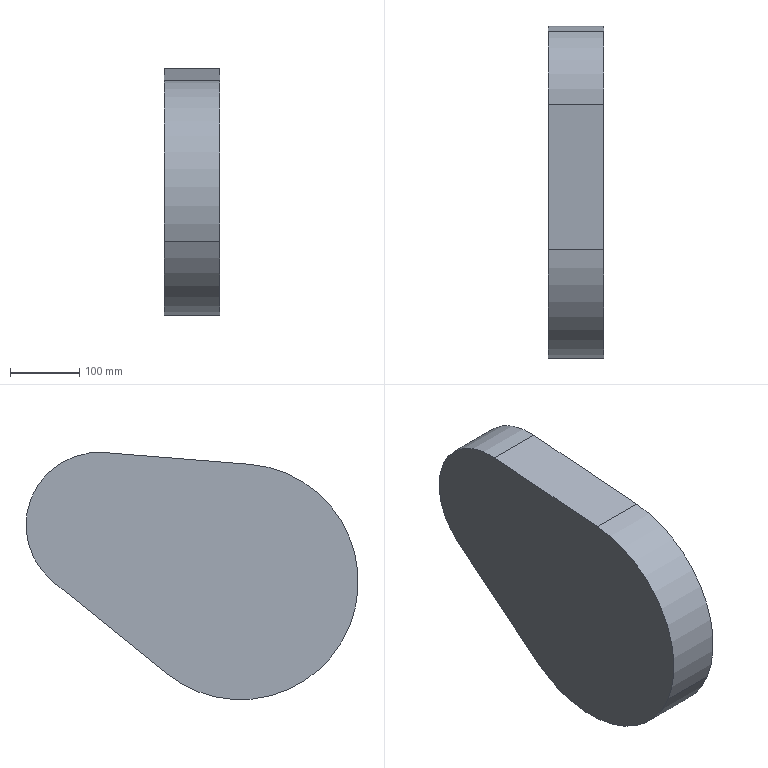Part | STEP file | Boss-Extrude 2 | 1 solid | 21 faces | box 80 x 479.268 x 356.697 mm | volume 2188971 mm3 | cylinder 12 | plane 9 | commonest cylinder face diameters 50 x2 60 x2 190 x2 210 x2 320 x2 340 x2
STEP:
#1=CARTESIAN_POINT('',(-70.976,-225.269,2449.643));
#2=VERTEX_POINT('',#1);
#3=CARTESIAN_POINT('',(-70.976,-196.827,2558.767));
#4=VERTEX_POINT('',#3);
#5=CARTESIAN_POINT('',(-70.976,-285.033,2523.489));
#6=DIRECTION('',(1.,0.,0.));
#7=DIRECTION('',(0.,0.9285,0.3713));
#8=AXIS2_PLACEMENT_3D('',#5,#6,#7);
#9=CIRCLE('',#8,95.);
#10=EDGE_CURVE('',#2,#4,#9,.T.);
#11=ORIENTED_EDGE('',*,*,#10,.T.);
#12=CARTESIAN_POINT('',(-140.976,-196.827,2558.767));
#13=VERTEX_POINT('',#12);
#14=CARTESIAN_POINT('',(-70.976,-196.827,2558.767));
#15=DIRECTION('',(-1.,0.,0.));
#16=VECTOR('',#15,1000.);
#17=LINE('',#14,#16);
#18=EDGE_CURVE('',#4,#13,#17,.T.);
#19=ORIENTED_EDGE('',*,*,#18,.T.);
#20=CARTESIAN_POINT('',(-140.976,-225.269,2449.643));
#21=VERTEX_POINT('',#20);
#22=CARTESIAN_POINT('',(-140.976,-285.033,2523.489));
#23=DIRECTION('',(1.,0.,0.));
#24=DIRECTION('',(0.,0.9285,0.3713));
#25=AXIS2_PLACEMENT_3D('',#22,#23,#24);
#26=CIRCLE('',#25,95.);
#27=EDGE_CURVE('',#21,#13,#26,.T.);
#28=ORIENTED_EDGE('',*,*,#27,.F.);
#29=CARTESIAN_POINT('',(-70.976,-225.269,2449.643));
#30=DIRECTION('',(-1.,0.,0.));
#31=VECTOR('',#30,1000.);
#32=LINE('',#29,#31);
#33=EDGE_CURVE('',#2,#21,#32,.T.);
#34=ORIENTED_EDGE('',*,*,#33,.F.);
#35=EDGE_LOOP('',(#11,#19,#28,#34));
#36=FACE_OUTER_BOUND('',#35,.T.);
#37=CARTESIAN_POINT('',(-70.976,-285.033,2523.489));
#38=DIRECTION('',(-1.,0.,0.));
#39=DIRECTION('',(0.,0.9285,0.3713));
#40=AXIS2_PLACEMENT_3D('',#37,#38,#39);
#41=CYLINDRICAL_SURFACE('',#40,95.);
#42=ADVANCED_FACE('',(#36),#41,.F.);
#43=CARTESIAN_POINT('',(-70.976,-187.542,2562.481));
#44=VERTEX_POINT('',#43);
#45=CARTESIAN_POINT('',(-70.976,-293.48,2628.149));
#46=VERTEX_POINT('',#45);
#47=CARTESIAN_POINT('',(-70.976,-285.033,2523.489));
#48=DIRECTION('',(1.,0.,0.));
#49=DIRECTION('',(0.,0.9285,0.3713));
#50=AXIS2_PLACEMENT_3D('',#47,#48,#49);
#51=CIRCLE('',#50,105.);
#52=EDGE_CURVE('',#44,#46,#51,.T.);
#53=ORIENTED_EDGE('',*,*,#52,.F.);
#54=CARTESIAN_POINT('',(-150.976,-187.542,2562.481));
#55=VERTEX_POINT('',#54);
#56=CARTESIAN_POINT('',(-70.976,-187.542,2562.481));
#57=DIRECTION('',(-1.,0.,0.));
#58=VECTOR('',#57,1000.);
#59=LINE('',#56,#58);
#60=EDGE_CURVE('',#44,#55,#59,.T.);
#61=ORIENTED_EDGE('',*,*,#60,.T.);
#62=CARTESIAN_POINT('',(-150.976,-293.48,2628.149));
#63=VERTEX_POINT('',#62);
#64=CARTESIAN_POINT('',(-150.976,-285.033,2523.489));
#65=DIRECTION('',(1.,0.,0.));
#66=DIRECTION('',(0.,0.9285,0.3713));
#67=AXIS2_PLACEMENT_3D('',#64,#65,#66);
#68=CIRCLE('',#67,105.);
#69=EDGE_CURVE('',#55,#63,#68,.T.);
#70=ORIENTED_EDGE('',*,*,#69,.T.);
#71=CARTESIAN_POINT('',(-70.976,-293.48,2628.149));
#72=DIRECTION('',(-1.,0.,0.));
#73=VECTOR('',#72,1000.);
#74=LINE('',#71,#73);
#75=EDGE_CURVE('',#46,#63,#74,.T.);
#76=ORIENTED_EDGE('',*,*,#75,.F.);
#77=EDGE_LOOP('',(#53,#61,#70,#76));
#78=FACE_OUTER_BOUND('',#77,.T.);
#79=CARTESIAN_POINT('',(-70.976,-285.033,2523.489));
#80=DIRECTION('',(-1.,0.,0.));
#81=DIRECTION('',(0.,0.9285,0.3713));
#82=AXIS2_PLACEMENT_3D('',#79,#80,#81);
#83=CYLINDRICAL_SURFACE('',#82,105.);
#84=ADVANCED_FACE('',(#78),#83,.T.);
#85=CARTESIAN_POINT('',(-110.976,-512.514,2432.508));
#86=VERTEX_POINT('',#85);
#87=CARTESIAN_POINT('',(-110.976,-466.089,2451.076));
#88=VERTEX_POINT('',#87);
#89=CARTESIAN_POINT('',(-110.976,-489.302,2441.792));
#90=DIRECTION('',(1.,0.,0.));
#91=DIRECTION('',(0.,0.9285,0.3713));
#92=AXIS2_PLACEMENT_3D('',#89,#90,#91);
#93=CIRCLE('',#92,25.);
#94=EDGE_CURVE('',#86,#88,#93,.T.);
#95=ORIENTED_EDGE('',*,*,#94,.T.);
#96=CARTESIAN_POINT('',(-140.976,-466.089,2451.076));
#97=VERTEX_POINT('',#96);
#98=CARTESIAN_POINT('',(-110.976,-466.089,2451.076));
#99=DIRECTION('',(1.,0.,0.));
#100=VECTOR('',#99,1000.);
#101=LINE('',#98,#100);
#102=EDGE_CURVE('',#97,#88,#101,.T.);
#103=ORIENTED_EDGE('',*,*,#102,.F.);
#104=CARTESIAN_POINT('',(-140.976,-512.514,2432.508));
#105=VERTEX_POINT('',#104);
#106=CARTESIAN_POINT('',(-140.976,-489.302,2441.792));
#107=DIRECTION('',(-1.,0.,0.));
#108=DIRECTION('',(0.,0.9285,0.3713));
#109=AXIS2_PLACEMENT_3D('',#106,#107,#108);
#110=CIRCLE('',#109,25.);
#111=EDGE_CURVE('',#97,#105,#110,.T.);
#112=ORIENTED_EDGE('',*,*,#111,.T.);
#113=CARTESIAN_POINT('',(-110.976,-512.514,2432.508));
#114=DIRECTION('',(1.,0.,0.));
#115=VECTOR('',#114,1000.);
#116=LINE('',#113,#115);
#117=EDGE_CURVE('',#105,#86,#116,.T.);
#118=ORIENTED_EDGE('',*,*,#117,.T.);
#119=EDGE_LOOP('',(#95,#103,#112,#118));
#120=FACE_OUTER_BOUND('',#119,.T.);
#121=CARTESIAN_POINT('',(-110.976,-489.302,2441.792));
#122=DIRECTION('',(-1.,0.,0.));
#123=DIRECTION('',(0.,0.9285,0.3713));
#124=AXIS2_PLACEMENT_3D('',#121,#122,#123);
#125=CYLINDRICAL_SURFACE('',#124,25.);
#126=ADVANCED_FACE('',(#120),#125,.F.);
#127=CARTESIAN_POINT('',(-110.976,-461.447,2452.933));
#128=VERTEX_POINT('',#127);
#129=CARTESIAN_POINT('',(-110.976,-517.157,2430.652));
#130=VERTEX_POINT('',#129);
#131=CARTESIAN_POINT('',(-110.976,-489.302,2441.792));
#132=DIRECTION('',(1.,0.,0.));
#133=DIRECTION('',(0.,0.9285,0.3713));
#134=AXIS2_PLACEMENT_3D('',#131,#132,#133);
#135=CIRCLE('',#134,30.);
#136=EDGE_CURVE('',#128,#130,#135,.T.);
#137=ORIENTED_EDGE('',*,*,#136,.F.);
#138=CARTESIAN_POINT('',(-140.976,-461.447,2452.933));
#139=VERTEX_POINT('',#138);
#140=CARTESIAN_POINT('',(-110.976,-461.447,2452.933));
#141=DIRECTION('',(1.,0.,0.));
#142=VECTOR('',#141,1000.);
#143=LINE('',#140,#142);
#144=EDGE_CURVE('',#139,#128,#143,.T.);
#145=ORIENTED_EDGE('',*,*,#144,.F.);
#146=CARTESIAN_POINT('',(-140.976,-517.157,2430.652));
#147=VERTEX_POINT('',#146);
#148=CARTESIAN_POINT('',(-140.976,-489.302,2441.792));
#149=DIRECTION('',(1.,0.,0.));
#150=DIRECTION('',(0.,0.9285,0.3713));
#151=AXIS2_PLACEMENT_3D('',#148,#149,#150);
#152=CIRCLE('',#151,30.);
#153=EDGE_CURVE('',#139,#147,#152,.T.);
#154=ORIENTED_EDGE('',*,*,#153,.T.);
#155=CARTESIAN_POINT('',(-110.976,-517.157,2430.652));
#156=DIRECTION('',(1.,0.,0.));
#157=VECTOR('',#156,1000.);
#158=LINE('',#155,#157);
#159=EDGE_CURVE('',#147,#130,#158,.T.);
#160=ORIENTED_EDGE('',*,*,#159,.T.);
#161=EDGE_LOOP('',(#137,#145,#154,#160));
#162=FACE_OUTER_BOUND('',#161,.T.);
#163=CARTESIAN_POINT('',(-110.976,-489.302,2441.792));
#164=DIRECTION('',(-1.,0.,0.));
#165=DIRECTION('',(0.,0.9285,0.3713));
#166=AXIS2_PLACEMENT_3D('',#163,#164,#165);
#167=CYLINDRICAL_SURFACE('',#166,30.);
#168=ADVANCED_FACE('',(#162),#167,.T.);
#169=CARTESIAN_POINT('',(-70.976,-502.173,2601.274));
#170=VERTEX_POINT('',#169);
#171=CARTESIAN_POINT('',(-70.976,-637.861,2382.376));
#172=VERTEX_POINT('',#171);
#173=CARTESIAN_POINT('',(-70.976,-489.302,2441.792));
#174=DIRECTION('',(1.,0.,0.));
#175=DIRECTION('',(0.,0.9285,0.3713));
#176=AXIS2_PLACEMENT_3D('',#173,#174,#175);
#177=CIRCLE('',#176,160.);
#178=EDGE_CURVE('',#170,#172,#177,.T.);
#179=ORIENTED_EDGE('',*,*,#178,.T.);
#180=CARTESIAN_POINT('',(-140.976,-637.861,2382.376));
#181=VERTEX_POINT('',#180);
#182=CARTESIAN_POINT('',(-70.976,-637.861,2382.376));
#183=DIRECTION('',(-1.,0.,0.));
#184=VECTOR('',#183,1000.);
#185=LINE('',#182,#184);
#186=EDGE_CURVE('',#172,#181,#185,.T.);
#187=ORIENTED_EDGE('',*,*,#186,.T.);
#188=CARTESIAN_POINT('',(-140.976,-502.173,2601.274));
#189=VERTEX_POINT('',#188);
#190=CARTESIAN_POINT('',(-140.976,-489.302,2441.792));
#191=DIRECTION('',(1.,0.,0.));
#192=DIRECTION('',(0.,0.9285,0.3713));
#193=AXIS2_PLACEMENT_3D('',#190,#191,#192);
#194=CIRCLE('',#193,160.);
#195=EDGE_CURVE('',#189,#181,#194,.T.);
#196=ORIENTED_EDGE('',*,*,#195,.F.);
#197=CARTESIAN_POINT('',(-70.976,-502.173,2601.274));
#198=DIRECTION('',(-1.,0.,0.));
#199=VECTOR('',#198,1000.);
#200=LINE('',#197,#199);
#201=EDGE_CURVE('',#170,#189,#200,.T.);
#202=ORIENTED_EDGE('',*,*,#201,.F.);
#203=EDGE_LOOP('',(#179,#187,#196,#202));
#204=FACE_OUTER_BOUND('',#203,.T.);
#205=CARTESIAN_POINT('',(-70.976,-489.302,2441.792));
#206=DIRECTION('',(-1.,0.,0.));
#207=DIRECTION('',(0.,0.9285,0.3713));
#208=AXIS2_PLACEMENT_3D('',#205,#206,#207);
#209=CYLINDRICAL_SURFACE('',#208,160.);
#210=ADVANCED_FACE('',(#204),#209,.F.);
#211=CARTESIAN_POINT('',(-70.976,-647.146,2378.663));
#212=VERTEX_POINT('',#211);
#213=CARTESIAN_POINT('',(-70.976,-382.355,2309.647));
#214=VERTEX_POINT('',#213);
#215=CARTESIAN_POINT('',(-70.976,-489.302,2441.792));
#216=DIRECTION('',(1.,0.,0.));
#217=DIRECTION('',(0.,0.9285,0.3713));
#218=AXIS2_PLACEMENT_3D('',#215,#216,#217);
#219=CIRCLE('',#218,170.);
#220=EDGE_CURVE('',#212,#214,#219,.T.);
#221=ORIENTED_EDGE('',*,*,#220,.F.);
#222=CARTESIAN_POINT('',(-150.976,-647.146,2378.663));
#223=VERTEX_POINT('',#222);
#224=CARTESIAN_POINT('',(-70.976,-647.146,2378.663));
#225=DIRECTION('',(-1.,0.,0.));
#226=VECTOR('',#225,1000.);
#227=LINE('',#224,#226);
#228=EDGE_CURVE('',#212,#223,#227,.T.);
#229=ORIENTED_EDGE('',*,*,#228,.T.);
#230=CARTESIAN_POINT('',(-150.976,-382.355,2309.647));
#231=VERTEX_POINT('',#230);
#232=CARTESIAN_POINT('',(-150.976,-489.302,2441.792));
#233=DIRECTION('',(1.,0.,0.));
#234=DIRECTION('',(0.,0.9285,0.3713));
#235=AXIS2_PLACEMENT_3D('',#232,#233,#234);
#236=CIRCLE('',#235,170.);
#237=EDGE_CURVE('',#223,#231,#236,.T.);
#238=ORIENTED_EDGE('',*,*,#237,.T.);
#239=CARTESIAN_POINT('',(-70.976,-382.355,2309.647));
#240=DIRECTION('',(-1.,0.,0.));
#241=VECTOR('',#240,1000.);
#242=LINE('',#239,#241);
#243=EDGE_CURVE('',#214,#231,#242,.T.);
#244=ORIENTED_EDGE('',*,*,#243,.F.);
#245=EDGE_LOOP('',(#221,#229,#238,#244));
#246=FACE_OUTER_BOUND('',#245,.T.);
#247=CARTESIAN_POINT('',(-70.976,-489.302,2441.792));
#248=DIRECTION('',(-1.,0.,0.));
#249=DIRECTION('',(0.,0.9285,0.3713));
#250=AXIS2_PLACEMENT_3D('',#247,#248,#249);
#251=CYLINDRICAL_SURFACE('',#250,170.);
#252=ADVANCED_FACE('',(#246),#251,.T.);
#253=ORIENTED_EDGE('',*,*,#60,.F.);
#254=CARTESIAN_POINT('',(-70.976,-218.978,2441.87));
#255=VERTEX_POINT('',#254);
#256=CARTESIAN_POINT('',(-70.976,-285.033,2523.489));
#257=DIRECTION('',(1.,0.,0.));
#258=DIRECTION('',(0.,0.9285,0.3713));
#259=AXIS2_PLACEMENT_3D('',#256,#257,#258);
#260=CIRCLE('',#259,105.);
#261=EDGE_CURVE('',#255,#44,#260,.T.);
#262=ORIENTED_EDGE('',*,*,#261,.F.);
#263=CARTESIAN_POINT('',(-150.976,-218.978,2441.87));
#264=VERTEX_POINT('',#263);
#265=CARTESIAN_POINT('',(-70.976,-218.978,2441.87));
#266=DIRECTION('',(-1.,0.,0.));
#267=VECTOR('',#266,1000.);
#268=LINE('',#265,#267);
#269=EDGE_CURVE('',#255,#264,#268,.T.);
#270=ORIENTED_EDGE('',*,*,#269,.T.);
#271=CARTESIAN_POINT('',(-150.976,-285.033,2523.489));
#272=DIRECTION('',(1.,0.,0.));
#273=DIRECTION('',(0.,0.9285,0.3713));
#274=AXIS2_PLACEMENT_3D('',#271,#272,#273);
#275=CIRCLE('',#274,105.);
#276=EDGE_CURVE('',#264,#55,#275,.T.);
#277=ORIENTED_EDGE('',*,*,#276,.T.);
#278=EDGE_LOOP('',(#253,#262,#270,#277));
#279=FACE_OUTER_BOUND('',#278,.T.);
#280=CARTESIAN_POINT('',(-70.976,-285.033,2523.489));
#281=DIRECTION('',(-1.,0.,0.));
#282=DIRECTION('',(0.,0.9285,0.3713));
#283=AXIS2_PLACEMENT_3D('',#280,#281,#282);
#284=CYLINDRICAL_SURFACE('',#283,105.);
#285=ADVANCED_FACE('',(#279),#284,.T.);
#286=CARTESIAN_POINT('',(-150.976,-502.977,2611.241));
#287=VERTEX_POINT('',#286);
#288=CARTESIAN_POINT('',(-150.976,-502.977,2611.241));
#289=DIRECTION('',(0.,-0.9968,-0.08044));
#290=VECTOR('',#289,1000.);
#291=LINE('',#288,#290);
#292=EDGE_CURVE('',#63,#287,#291,.T.);
#293=ORIENTED_EDGE('',*,*,#292,.T.);
#294=CARTESIAN_POINT('',(-70.976,-502.977,2611.241));
#295=VERTEX_POINT('',#294);
#296=CARTESIAN_POINT('',(-70.976,-502.977,2611.241));
#297=DIRECTION('',(-1.,0.,0.));
#298=VECTOR('',#297,1000.);
#299=LINE('',#296,#298);
#300=EDGE_CURVE('',#295,#287,#299,.T.);
#301=ORIENTED_EDGE('',*,*,#300,.F.);
#302=CARTESIAN_POINT('',(-70.976,-502.977,2611.241));
#303=DIRECTION('',(0.,-0.9968,-0.08044));
#304=VECTOR('',#303,1000.);
#305=LINE('',#302,#304);
#306=EDGE_CURVE('',#46,#295,#305,.T.);
#307=ORIENTED_EDGE('',*,*,#306,.F.);
#308=ORIENTED_EDGE('',*,*,#75,.T.);
#309=EDGE_LOOP('',(#293,#301,#307,#308));
#310=FACE_OUTER_BOUND('',#309,.T.);
#311=CARTESIAN_POINT('',(-70.976,-502.977,2611.241));
#312=DIRECTION('',(0.,0.08044,-0.9968));
#313=DIRECTION('',(0.,-0.9968,-0.08044));
#314=AXIS2_PLACEMENT_3D('',#311,#312,#313);
#315=PLANE('',#314);
#316=ADVANCED_FACE('',(#310),#315,.F.);
#317=ORIENTED_EDGE('',*,*,#228,.F.);
#318=CARTESIAN_POINT('',(-70.976,-489.302,2441.792));
#319=DIRECTION('',(1.,0.,0.));
#320=DIRECTION('',(0.,0.9285,0.3713));
#321=AXIS2_PLACEMENT_3D('',#318,#319,#320);
#322=CIRCLE('',#321,170.);
#323=EDGE_CURVE('',#295,#212,#322,.T.);
#324=ORIENTED_EDGE('',*,*,#323,.F.);
#325=ORIENTED_EDGE('',*,*,#300,.T.);
#326=CARTESIAN_POINT('',(-150.976,-489.302,2441.792));
#327=DIRECTION('',(1.,0.,0.));
#328=DIRECTION('',(0.,0.9285,0.3713));
#329=AXIS2_PLACEMENT_3D('',#326,#327,#328);
#330=CIRCLE('',#329,170.);
#331=EDGE_CURVE('',#287,#223,#330,.T.);
#332=ORIENTED_EDGE('',*,*,#331,.T.);
#333=EDGE_LOOP('',(#317,#324,#325,#332));
#334=FACE_OUTER_BOUND('',#333,.T.);
#335=CARTESIAN_POINT('',(-70.976,-489.302,2441.792));
#336=DIRECTION('',(-1.,0.,0.));
#337=DIRECTION('',(0.,0.9285,0.3713));
#338=AXIS2_PLACEMENT_3D('',#335,#336,#337);
#339=CYLINDRICAL_SURFACE('',#338,170.);
#340=ADVANCED_FACE('',(#334),#339,.T.);
#341=CARTESIAN_POINT('',(-150.976,-382.355,2309.647));
#342=DIRECTION('',(0.,0.7773,0.6291));
#343=VECTOR('',#342,1000.);
#344=LINE('',#341,#343);
#345=EDGE_CURVE('',#231,#264,#344,.T.);
#346=ORIENTED_EDGE('',*,*,#345,.T.);
#347=ORIENTED_EDGE('',*,*,#269,.F.);
#348=CARTESIAN_POINT('',(-70.976,-382.355,2309.647));
#349=DIRECTION('',(0.,0.7773,0.6291));
#350=VECTOR('',#349,1000.);
#351=LINE('',#348,#350);
#352=EDGE_CURVE('',#214,#255,#351,.T.);
#353=ORIENTED_EDGE('',*,*,#352,.F.);
#354=ORIENTED_EDGE('',*,*,#243,.T.);
#355=EDGE_LOOP('',(#346,#347,#353,#354));
#356=FACE_OUTER_BOUND('',#355,.T.);
#357=CARTESIAN_POINT('',(-70.976,-382.355,2309.647));
#358=DIRECTION('',(0.,-0.6291,0.7773));
#359=DIRECTION('',(0.,0.7773,0.6291));
#360=AXIS2_PLACEMENT_3D('',#357,#358,#359);
#361=PLANE('',#360);
#362=ADVANCED_FACE('',(#356),#361,.F.);
#363=ORIENTED_EDGE('',*,*,#10,.F.);
#364=CARTESIAN_POINT('',(-70.976,-388.646,2317.42));
#365=VERTEX_POINT('',#364);
#366=CARTESIAN_POINT('',(-70.976,-388.646,2317.42));
#367=DIRECTION('',(0.,0.7773,0.6291));
#368=VECTOR('',#367,1000.);
#369=LINE('',#366,#368);
#370=EDGE_CURVE('',#365,#2,#369,.T.);
#371=ORIENTED_EDGE('',*,*,#370,.F.);
#372=CARTESIAN_POINT('',(-70.976,-489.302,2441.792));
#373=DIRECTION('',(1.,0.,0.));
#374=DIRECTION('',(0.,0.9285,0.3713));
#375=AXIS2_PLACEMENT_3D('',#372,#373,#374);
#376=CIRCLE('',#375,160.);
#377=EDGE_CURVE('',#172,#365,#376,.T.);
#378=ORIENTED_EDGE('',*,*,#377,.F.);
#379=ORIENTED_EDGE('',*,*,#178,.F.);
#380=CARTESIAN_POINT('',(-70.976,-292.676,2618.181));
#381=VERTEX_POINT('',#380);
#382=CARTESIAN_POINT('',(-70.976,-502.173,2601.274));
#383=DIRECTION('',(0.,-0.9968,-0.08044));
#384=VECTOR('',#383,1000.);
#385=LINE('',#382,#384);
#386=EDGE_CURVE('',#381,#170,#385,.T.);
#387=ORIENTED_EDGE('',*,*,#386,.F.);
#388=CARTESIAN_POINT('',(-70.976,-285.033,2523.489));
#389=DIRECTION('',(1.,0.,0.));
#390=DIRECTION('',(0.,0.9285,0.3713));
#391=AXIS2_PLACEMENT_3D('',#388,#389,#390);
#392=CIRCLE('',#391,95.);
#393=EDGE_CURVE('',#4,#381,#392,.T.);
#394=ORIENTED_EDGE('',*,*,#393,.F.);
#395=EDGE_LOOP('',(#363,#371,#378,#379,#387,#394));
#396=FACE_BOUND('',#395,.T.);
#397=ORIENTED_EDGE('',*,*,#261,.T.);
#398=ORIENTED_EDGE('',*,*,#52,.T.);
#399=ORIENTED_EDGE('',*,*,#306,.T.);
#400=ORIENTED_EDGE('',*,*,#323,.T.);
#401=ORIENTED_EDGE('',*,*,#220,.T.);
#402=ORIENTED_EDGE('',*,*,#352,.T.);
#403=EDGE_LOOP('',(#397,#398,#399,#400,#401,#402));
#404=FACE_OUTER_BOUND('',#403,.T.);
#405=CARTESIAN_POINT('',(-70.976,-285.033,2523.489));
#406=DIRECTION('',(1.,0.,0.));
#407=DIRECTION('',(0.,-0.9285,-0.3713));
#408=AXIS2_PLACEMENT_3D('',#405,#406,#407);
#409=PLANE('',#408);
#410=ADVANCED_FACE('',(#396,#404),#409,.T.);
#411=ORIENTED_EDGE('',*,*,#276,.F.);
#412=ORIENTED_EDGE('',*,*,#345,.F.);
#413=ORIENTED_EDGE('',*,*,#237,.F.);
#414=ORIENTED_EDGE('',*,*,#331,.F.);
#415=ORIENTED_EDGE('',*,*,#292,.F.);
#416=ORIENTED_EDGE('',*,*,#69,.F.);
#417=EDGE_LOOP('',(#411,#412,#413,#414,#415,#416));
#418=FACE_OUTER_BOUND('',#417,.T.);
#419=CARTESIAN_POINT('',(-150.976,-285.033,2523.489));
#420=DIRECTION('',(1.,0.,0.));
#421=DIRECTION('',(0.,-0.9285,-0.3713));
#422=AXIS2_PLACEMENT_3D('',#419,#420,#421);
#423=PLANE('',#422);
#424=ADVANCED_FACE('',(#418),#423,.F.);
#425=ORIENTED_EDGE('',*,*,#18,.F.);
#426=ORIENTED_EDGE('',*,*,#393,.T.);
#427=CARTESIAN_POINT('',(-140.976,-292.676,2618.181));
#428=VERTEX_POINT('',#427);
#429=CARTESIAN_POINT('',(-70.976,-292.676,2618.181));
#430=DIRECTION('',(-1.,0.,0.));
#431=VECTOR('',#430,1000.);
#432=LINE('',#429,#431);
#433=EDGE_CURVE('',#381,#428,#432,.T.);
#434=ORIENTED_EDGE('',*,*,#433,.T.);
#435=CARTESIAN_POINT('',(-140.976,-285.033,2523.489));
#436=DIRECTION('',(1.,0.,0.));
#437=DIRECTION('',(0.,0.9285,0.3713));
#438=AXIS2_PLACEMENT_3D('',#435,#436,#437);
#439=CIRCLE('',#438,95.);
#440=EDGE_CURVE('',#13,#428,#439,.T.);
#441=ORIENTED_EDGE('',*,*,#440,.F.);
#442=EDGE_LOOP('',(#425,#426,#434,#441));
#443=FACE_OUTER_BOUND('',#442,.T.);
#444=CARTESIAN_POINT('',(-70.976,-285.033,2523.489));
#445=DIRECTION('',(-1.,0.,0.));
#446=DIRECTION('',(0.,0.9285,0.3713));
#447=AXIS2_PLACEMENT_3D('',#444,#445,#446);
#448=CYLINDRICAL_SURFACE('',#447,95.);
#449=ADVANCED_FACE('',(#443),#448,.F.);
#450=CARTESIAN_POINT('',(-140.976,-502.173,2601.274));
#451=DIRECTION('',(0.,-0.9968,-0.08044));
#452=VECTOR('',#451,1000.);
#453=LINE('',#450,#452);
#454=EDGE_CURVE('',#428,#189,#453,.T.);
#455=ORIENTED_EDGE('',*,*,#454,.F.);
#456=ORIENTED_EDGE('',*,*,#433,.F.);
#457=ORIENTED_EDGE('',*,*,#386,.T.);
#458=ORIENTED_EDGE('',*,*,#201,.T.);
#459=EDGE_LOOP('',(#455,#456,#457,#458));
#460=FACE_OUTER_BOUND('',#459,.T.);
#461=CARTESIAN_POINT('',(-70.976,-502.173,2601.274));
#462=DIRECTION('',(0.,0.08044,-0.9968));
#463=DIRECTION('',(0.,-0.9968,-0.08044));
#464=AXIS2_PLACEMENT_3D('',#461,#462,#463);
#465=PLANE('',#464);
#466=ADVANCED_FACE('',(#460),#465,.T.);
#467=ORIENTED_EDGE('',*,*,#186,.F.);
#468=ORIENTED_EDGE('',*,*,#377,.T.);
#469=CARTESIAN_POINT('',(-140.976,-388.646,2317.42));
#470=VERTEX_POINT('',#469);
#471=CARTESIAN_POINT('',(-70.976,-388.646,2317.42));
#472=DIRECTION('',(-1.,0.,0.));
#473=VECTOR('',#472,1000.);
#474=LINE('',#471,#473);
#475=EDGE_CURVE('',#365,#470,#474,.T.);
#476=ORIENTED_EDGE('',*,*,#475,.T.);
#477=CARTESIAN_POINT('',(-140.976,-489.302,2441.792));
#478=DIRECTION('',(1.,0.,0.));
#479=DIRECTION('',(0.,0.9285,0.3713));
#480=AXIS2_PLACEMENT_3D('',#477,#478,#479);
#481=CIRCLE('',#480,160.);
#482=EDGE_CURVE('',#181,#470,#481,.T.);
#483=ORIENTED_EDGE('',*,*,#482,.F.);
#484=EDGE_LOOP('',(#467,#468,#476,#483));
#485=FACE_OUTER_BOUND('',#484,.T.);
#486=CARTESIAN_POINT('',(-70.976,-489.302,2441.792));
#487=DIRECTION('',(-1.,0.,0.));
#488=DIRECTION('',(0.,0.9285,0.3713));
#489=AXIS2_PLACEMENT_3D('',#486,#487,#488);
#490=CYLINDRICAL_SURFACE('',#489,160.);
#491=ADVANCED_FACE('',(#485),#490,.F.);
#492=CARTESIAN_POINT('',(-140.976,-388.646,2317.42));
#493=DIRECTION('',(0.,0.7773,0.6291));
#494=VECTOR('',#493,1000.);
#495=LINE('',#492,#494);
#496=EDGE_CURVE('',#470,#21,#495,.T.);
#497=ORIENTED_EDGE('',*,*,#496,.F.);
#498=ORIENTED_EDGE('',*,*,#475,.F.);
#499=ORIENTED_EDGE('',*,*,#370,.T.);
#500=ORIENTED_EDGE('',*,*,#33,.T.);
#501=EDGE_LOOP('',(#497,#498,#499,#500));
#502=FACE_OUTER_BOUND('',#501,.T.);
#503=CARTESIAN_POINT('',(-70.976,-388.646,2317.42));
#504=DIRECTION('',(0.,-0.6291,0.7773));
#505=DIRECTION('',(0.,0.7773,0.6291));
#506=AXIS2_PLACEMENT_3D('',#503,#504,#505);
#507=PLANE('',#506);
#508=ADVANCED_FACE('',(#502),#507,.T.);
#509=CARTESIAN_POINT('',(-140.976,-489.302,2441.792));
#510=DIRECTION('',(1.,0.,0.));
#511=DIRECTION('',(0.,0.9285,0.3713));
#512=AXIS2_PLACEMENT_3D('',#509,#510,#511);
#513=CIRCLE('',#512,30.);
#514=EDGE_CURVE('',#147,#139,#513,.T.);
#515=ORIENTED_EDGE('',*,*,#514,.F.);
#516=ORIENTED_EDGE('',*,*,#153,.F.);
#517=EDGE_LOOP('',(#515,#516));
#518=FACE_BOUND('',#517,.T.);
#519=ORIENTED_EDGE('',*,*,#27,.T.);
#520=ORIENTED_EDGE('',*,*,#440,.T.);
#521=ORIENTED_EDGE('',*,*,#454,.T.);
#522=ORIENTED_EDGE('',*,*,#195,.T.);
#523=ORIENTED_EDGE('',*,*,#482,.T.);
#524=ORIENTED_EDGE('',*,*,#496,.T.);
#525=EDGE_LOOP('',(#519,#520,#521,#522,#523,#524));
#526=FACE_OUTER_BOUND('',#525,.T.);
#527=CARTESIAN_POINT('',(-140.976,-285.033,2523.489));
#528=DIRECTION('',(1.,0.,0.));
#529=DIRECTION('',(0.,-0.9285,-0.3713));
#530=AXIS2_PLACEMENT_3D('',#527,#528,#529);
#531=PLANE('',#530);
#532=ADVANCED_FACE('',(#518,#526),#531,.T.);
#533=CARTESIAN_POINT('',(-110.976,-489.302,2441.792));
#534=DIRECTION('',(1.,0.,0.));
#535=DIRECTION('',(0.,0.9285,0.3713));
#536=AXIS2_PLACEMENT_3D('',#533,#534,#535);
#537=CIRCLE('',#536,30.);
#538=EDGE_CURVE('',#130,#128,#537,.T.);
#539=ORIENTED_EDGE('',*,*,#538,.T.);
#540=ORIENTED_EDGE('',*,*,#136,.T.);
#541=EDGE_LOOP('',(#539,#540));
#542=FACE_OUTER_BOUND('',#541,.T.);
#543=ORIENTED_EDGE('',*,*,#94,.F.);
#544=CARTESIAN_POINT('',(-110.976,-489.302,2441.792));
#545=DIRECTION('',(1.,0.,0.));
#546=DIRECTION('',(0.,0.9285,0.3713));
#547=AXIS2_PLACEMENT_3D('',#544,#545,#546);
#548=CIRCLE('',#547,25.);
#549=EDGE_CURVE('',#88,#86,#548,.T.);
#550=ORIENTED_EDGE('',*,*,#549,.F.);
#551=EDGE_LOOP('',(#543,#550));
#552=FACE_BOUND('',#551,.T.);
#553=CARTESIAN_POINT('',(-110.976,-489.302,2441.792));
#554=DIRECTION('',(1.,0.,0.));
#555=DIRECTION('',(0.,-0.9285,-0.3713));
#556=AXIS2_PLACEMENT_3D('',#553,#554,#555);
#557=PLANE('',#556);
#558=ADVANCED_FACE('',(#542,#552),#557,.T.);
#559=ORIENTED_EDGE('',*,*,#144,.T.);
#560=ORIENTED_EDGE('',*,*,#538,.F.);
#561=ORIENTED_EDGE('',*,*,#159,.F.);
#562=ORIENTED_EDGE('',*,*,#514,.T.);
#563=EDGE_LOOP('',(#559,#560,#561,#562));
#564=FACE_OUTER_BOUND('',#563,.T.);
#565=CARTESIAN_POINT('',(-110.976,-489.302,2441.792));
#566=DIRECTION('',(-1.,0.,0.));
#567=DIRECTION('',(0.,0.9285,0.3713));
#568=AXIS2_PLACEMENT_3D('',#565,#566,#567);
#569=CYLINDRICAL_SURFACE('',#568,30.);
#570=ADVANCED_FACE('',(#564),#569,.T.);
#571=ORIENTED_EDGE('',*,*,#102,.T.);
#572=ORIENTED_EDGE('',*,*,#549,.T.);
#573=ORIENTED_EDGE('',*,*,#117,.F.);
#574=CARTESIAN_POINT('',(-140.976,-489.302,2441.792));
#575=DIRECTION('',(-1.,0.,0.));
#576=DIRECTION('',(0.,0.9285,0.3713));
#577=AXIS2_PLACEMENT_3D('',#574,#575,#576);
#578=CIRCLE('',#577,25.);
#579=EDGE_CURVE('',#105,#97,#578,.T.);
#580=ORIENTED_EDGE('',*,*,#579,.T.);
#581=EDGE_LOOP('',(#571,#572,#573,#580));
#582=FACE_OUTER_BOUND('',#581,.T.);
#583=CARTESIAN_POINT('',(-110.976,-489.302,2441.792));
#584=DIRECTION('',(-1.,0.,0.));
#585=DIRECTION('',(0.,0.9285,0.3713));
#586=AXIS2_PLACEMENT_3D('',#583,#584,#585);
#587=CYLINDRICAL_SURFACE('',#586,25.);
#588=ADVANCED_FACE('',(#582),#587,.F.);
#589=ORIENTED_EDGE('',*,*,#579,.F.);
#590=ORIENTED_EDGE('',*,*,#111,.F.);
#591=EDGE_LOOP('',(#589,#590));
#592=FACE_OUTER_BOUND('',#591,.T.);
#593=CARTESIAN_POINT('',(-140.976,-285.033,2523.489));
#594=DIRECTION('',(1.,0.,0.));
#595=DIRECTION('',(0.,-0.9285,-0.3713));
#596=AXIS2_PLACEMENT_3D('',#593,#594,#595);
#597=PLANE('',#596);
#598=ADVANCED_FACE('',(#592),#597,.T.);
#599=CLOSED_SHELL('',(#42,#84,#126,#168,#210,#252,#285,#316,#340,#362,#410,#424,#449,#466,#491,#508,#532,#558,#570,#588,#598));
#600=MANIFOLD_SOLID_BREP('',#599);
#601=CARTESIAN_POINT('',(0.,0.,0.));
#602=DIRECTION('',(0.,0.,1.));
#603=DIRECTION('',(1.,0.,0.));
#604=AXIS2_PLACEMENT_3D('',#601,#602,#603);
#605=(LENGTH_UNIT()NAMED_UNIT(*)SI_UNIT(.MILLI.,.METRE.));
#606=UNCERTAINTY_MEASURE_WITH_UNIT(LENGTH_MEASURE(0.00001),#605,'','');
#607=(NAMED_UNIT(*)PLANE_ANGLE_UNIT()SI_UNIT($,.RADIAN.));
#608=(NAMED_UNIT(*)SI_UNIT($,.STERADIAN.)SOLID_ANGLE_UNIT());
#609=(GEOMETRIC_REPRESENTATION_CONTEXT(3)GLOBAL_UNCERTAINTY_ASSIGNED_CONTEXT((#606))GLOBAL_UNIT_ASSIGNED_CONTEXT((#605,#607,#608))REPRESENTATION_CONTEXT('',''));
#610=ADVANCED_BREP_SHAPE_REPRESENTATION('',(#600,#604),#609);